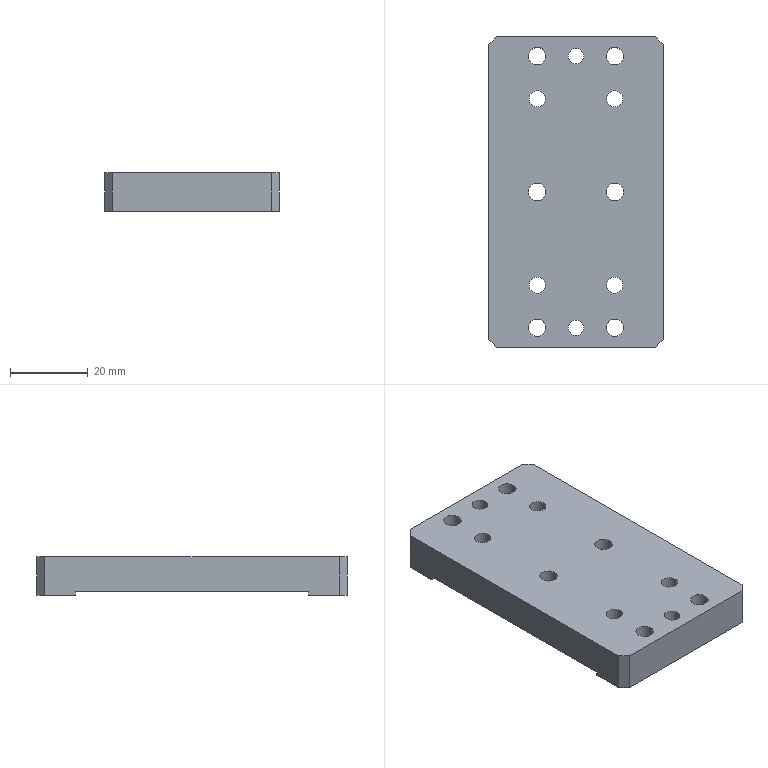Part | STEP file | PN_0052 Mount electronic clip manipulator mounting plate | 1 solid | 56 faces | box 45 x 80 x 10 mm | volume 30659 mm3 | cylinder 36 | plane 20 | commonest cylinder face diameters 4.5 x12 8 x12 4.2 x8 4 x4